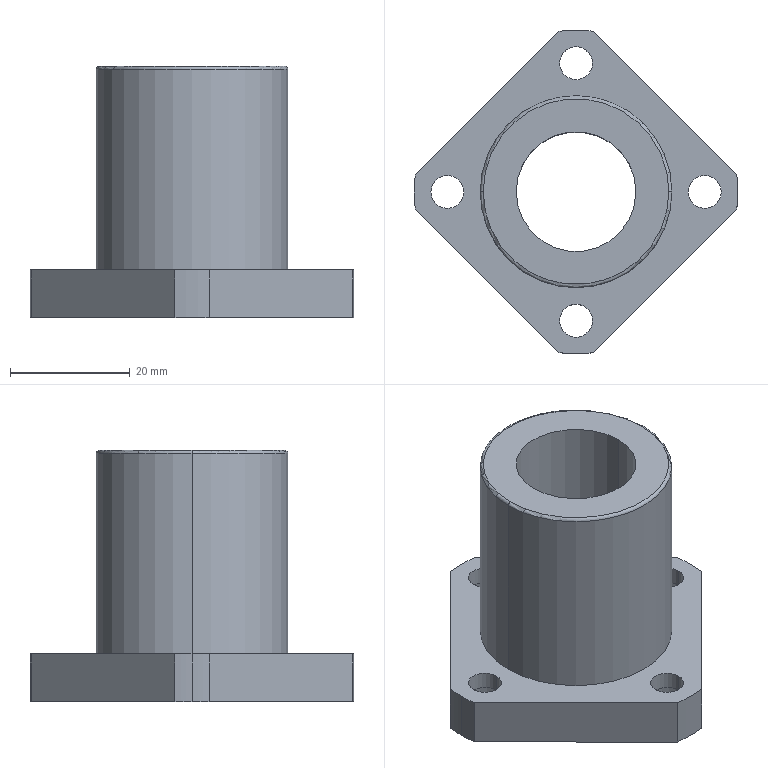Part | SolidWorks | features BaseBody 1 | 1 solid | 38 faces | box 54 x 54 x 42 mm | volume 26442 mm3 | cylinder 25 | plane 11 | torus 2 | commonest cylinder face diameters 5.5 x8 9 x8 54 x5 20 x2 32 x2
STEP:
#1=CARTESIAN_POINT('',(4.5,21.5,5.1));
#2=VERTEX_POINT('',#1);
#3=CARTESIAN_POINT('',(-4.5,21.5,5.1));
#4=VERTEX_POINT('',#3);
#5=CARTESIAN_POINT('',(0.,21.5,5.1));
#6=DIRECTION('',(0.,0.,-1.));
#7=DIRECTION('',(-1.,0.,0.));
#8=AXIS2_PLACEMENT_3D('',#5,#6,#7);
#9=CIRCLE('',#8,4.5);
#10=EDGE_CURVE('',#2,#4,#9,.T.);
#11=ORIENTED_EDGE('',*,*,#10,.F.);
#12=CARTESIAN_POINT('',(4.5,21.5,0.));
#13=VERTEX_POINT('',#12);
#14=CARTESIAN_POINT('',(4.5,21.5,0.));
#15=DIRECTION('',(0.,0.,-1.));
#16=VECTOR('',#15,1000.);
#17=LINE('',#14,#16);
#18=EDGE_CURVE('',#2,#13,#17,.T.);
#19=ORIENTED_EDGE('',*,*,#18,.T.);
#20=CARTESIAN_POINT('',(-4.5,21.5,0.));
#21=VERTEX_POINT('',#20);
#22=CARTESIAN_POINT('',(0.,21.5,0.));
#23=DIRECTION('',(0.,0.,-1.));
#24=DIRECTION('',(-1.,0.,0.));
#25=AXIS2_PLACEMENT_3D('',#22,#23,#24);
#26=CIRCLE('',#25,4.5);
#27=EDGE_CURVE('',#13,#21,#26,.T.);
#28=ORIENTED_EDGE('',*,*,#27,.T.);
#29=CARTESIAN_POINT('',(-4.5,21.5,0.));
#30=DIRECTION('',(0.,0.,-1.));
#31=VECTOR('',#30,1000.);
#32=LINE('',#29,#31);
#33=EDGE_CURVE('',#4,#21,#32,.T.);
#34=ORIENTED_EDGE('',*,*,#33,.F.);
#35=EDGE_LOOP('',(#11,#19,#28,#34));
#36=FACE_OUTER_BOUND('',#35,.T.);
#37=CARTESIAN_POINT('',(0.,21.5,0.));
#38=DIRECTION('',(0.,0.,-1.));
#39=DIRECTION('',(-1.,0.,0.));
#40=AXIS2_PLACEMENT_3D('',#37,#38,#39);
#41=CYLINDRICAL_SURFACE('',#40,4.5);
#42=ADVANCED_FACE('',(#36),#41,.F.);
#43=CARTESIAN_POINT('',(2.75,21.5,8.));
#44=VERTEX_POINT('',#43);
#45=CARTESIAN_POINT('',(-2.75,21.5,8.));
#46=VERTEX_POINT('',#45);
#47=CARTESIAN_POINT('',(0.,21.5,8.));
#48=DIRECTION('',(0.,0.,-1.));
#49=DIRECTION('',(-1.,0.,0.));
#50=AXIS2_PLACEMENT_3D('',#47,#48,#49);
#51=CIRCLE('',#50,2.75);
#52=EDGE_CURVE('',#44,#46,#51,.T.);
#53=ORIENTED_EDGE('',*,*,#52,.F.);
#54=CARTESIAN_POINT('',(2.75,21.5,5.1));
#55=VERTEX_POINT('',#54);
#56=CARTESIAN_POINT('',(2.75,21.5,0.));
#57=DIRECTION('',(0.,0.,-1.));
#58=VECTOR('',#57,1000.);
#59=LINE('',#56,#58);
#60=EDGE_CURVE('',#44,#55,#59,.T.);
#61=ORIENTED_EDGE('',*,*,#60,.T.);
#62=CARTESIAN_POINT('',(-2.75,21.5,5.1));
#63=VERTEX_POINT('',#62);
#64=CARTESIAN_POINT('',(0.,21.5,5.1));
#65=DIRECTION('',(0.,0.,-1.));
#66=DIRECTION('',(-1.,0.,0.));
#67=AXIS2_PLACEMENT_3D('',#64,#65,#66);
#68=CIRCLE('',#67,2.75);
#69=EDGE_CURVE('',#55,#63,#68,.T.);
#70=ORIENTED_EDGE('',*,*,#69,.T.);
#71=CARTESIAN_POINT('',(-2.75,21.5,0.));
#72=DIRECTION('',(0.,0.,-1.));
#73=VECTOR('',#72,1000.);
#74=LINE('',#71,#73);
#75=EDGE_CURVE('',#46,#63,#74,.T.);
#76=ORIENTED_EDGE('',*,*,#75,.F.);
#77=EDGE_LOOP('',(#53,#61,#70,#76));
#78=FACE_OUTER_BOUND('',#77,.T.);
#79=CARTESIAN_POINT('',(0.,21.5,0.));
#80=DIRECTION('',(0.,0.,-1.));
#81=DIRECTION('',(-1.,0.,0.));
#82=AXIS2_PLACEMENT_3D('',#79,#80,#81);
#83=CYLINDRICAL_SURFACE('',#82,2.75);
#84=ADVANCED_FACE('',(#78),#83,.F.);
#85=CARTESIAN_POINT('',(-2.75,-21.5,5.1));
#86=VERTEX_POINT('',#85);
#87=CARTESIAN_POINT('',(2.75,-21.5,5.1));
#88=VERTEX_POINT('',#87);
#89=CARTESIAN_POINT('',(0.,-21.5,5.1));
#90=DIRECTION('',(0.,0.,1.));
#91=DIRECTION('',(1.,0.,0.));
#92=AXIS2_PLACEMENT_3D('',#89,#90,#91);
#93=CIRCLE('',#92,2.75);
#94=EDGE_CURVE('',#86,#88,#93,.T.);
#95=ORIENTED_EDGE('',*,*,#94,.F.);
#96=CARTESIAN_POINT('',(-2.75,-21.5,8.));
#97=VERTEX_POINT('',#96);
#98=CARTESIAN_POINT('',(-2.75,-21.5,8.));
#99=DIRECTION('',(0.,0.,1.));
#100=VECTOR('',#99,1000.);
#101=LINE('',#98,#100);
#102=EDGE_CURVE('',#86,#97,#101,.T.);
#103=ORIENTED_EDGE('',*,*,#102,.T.);
#104=CARTESIAN_POINT('',(2.75,-21.5,8.));
#105=VERTEX_POINT('',#104);
#106=CARTESIAN_POINT('',(0.,-21.5,8.));
#107=DIRECTION('',(0.,0.,1.));
#108=DIRECTION('',(1.,0.,0.));
#109=AXIS2_PLACEMENT_3D('',#106,#107,#108);
#110=CIRCLE('',#109,2.75);
#111=EDGE_CURVE('',#97,#105,#110,.T.);
#112=ORIENTED_EDGE('',*,*,#111,.T.);
#113=CARTESIAN_POINT('',(2.75,-21.5,8.));
#114=DIRECTION('',(0.,0.,1.));
#115=VECTOR('',#114,1000.);
#116=LINE('',#113,#115);
#117=EDGE_CURVE('',#88,#105,#116,.T.);
#118=ORIENTED_EDGE('',*,*,#117,.F.);
#119=EDGE_LOOP('',(#95,#103,#112,#118));
#120=FACE_OUTER_BOUND('',#119,.T.);
#121=CARTESIAN_POINT('',(0.,-21.5,8.));
#122=DIRECTION('',(0.,0.,1.));
#123=DIRECTION('',(1.,0.,0.));
#124=AXIS2_PLACEMENT_3D('',#121,#122,#123);
#125=CYLINDRICAL_SURFACE('',#124,2.75);
#126=ADVANCED_FACE('',(#120),#125,.F.);
#127=CARTESIAN_POINT('',(-4.5,-21.5,0.));
#128=VERTEX_POINT('',#127);
#129=CARTESIAN_POINT('',(4.5,-21.5,0.));
#130=VERTEX_POINT('',#129);
#131=CARTESIAN_POINT('',(0.,-21.5,0.));
#132=DIRECTION('',(0.,0.,1.));
#133=DIRECTION('',(1.,0.,0.));
#134=AXIS2_PLACEMENT_3D('',#131,#132,#133);
#135=CIRCLE('',#134,4.5);
#136=EDGE_CURVE('',#128,#130,#135,.T.);
#137=ORIENTED_EDGE('',*,*,#136,.F.);
#138=CARTESIAN_POINT('',(-4.5,-21.5,5.1));
#139=VERTEX_POINT('',#138);
#140=CARTESIAN_POINT('',(-4.5,-21.5,8.));
#141=DIRECTION('',(0.,0.,1.));
#142=VECTOR('',#141,1000.);
#143=LINE('',#140,#142);
#144=EDGE_CURVE('',#128,#139,#143,.T.);
#145=ORIENTED_EDGE('',*,*,#144,.T.);
#146=CARTESIAN_POINT('',(4.5,-21.5,5.1));
#147=VERTEX_POINT('',#146);
#148=CARTESIAN_POINT('',(0.,-21.5,5.1));
#149=DIRECTION('',(0.,0.,1.));
#150=DIRECTION('',(1.,0.,0.));
#151=AXIS2_PLACEMENT_3D('',#148,#149,#150);
#152=CIRCLE('',#151,4.5);
#153=EDGE_CURVE('',#139,#147,#152,.T.);
#154=ORIENTED_EDGE('',*,*,#153,.T.);
#155=CARTESIAN_POINT('',(4.5,-21.5,8.));
#156=DIRECTION('',(0.,0.,1.));
#157=VECTOR('',#156,1000.);
#158=LINE('',#155,#157);
#159=EDGE_CURVE('',#130,#147,#158,.T.);
#160=ORIENTED_EDGE('',*,*,#159,.F.);
#161=EDGE_LOOP('',(#137,#145,#154,#160));
#162=FACE_OUTER_BOUND('',#161,.T.);
#163=CARTESIAN_POINT('',(0.,-21.5,8.));
#164=DIRECTION('',(0.,0.,1.));
#165=DIRECTION('',(1.,0.,0.));
#166=AXIS2_PLACEMENT_3D('',#163,#164,#165);
#167=CYLINDRICAL_SURFACE('',#166,4.5);
#168=ADVANCED_FACE('',(#162),#167,.F.);
#169=CARTESIAN_POINT('',(18.75,0.,5.1));
#170=VERTEX_POINT('',#169);
#171=CARTESIAN_POINT('',(24.25,0.,5.1));
#172=VERTEX_POINT('',#171);
#173=CARTESIAN_POINT('',(21.5,0.,5.1));
#174=DIRECTION('',(0.,0.,1.));
#175=DIRECTION('',(1.,0.,0.));
#176=AXIS2_PLACEMENT_3D('',#173,#174,#175);
#177=CIRCLE('',#176,2.75);
#178=EDGE_CURVE('',#170,#172,#177,.T.);
#179=ORIENTED_EDGE('',*,*,#178,.F.);
#180=CARTESIAN_POINT('',(18.75,0.,8.));
#181=VERTEX_POINT('',#180);
#182=CARTESIAN_POINT('',(18.75,0.,8.));
#183=DIRECTION('',(0.,0.,1.));
#184=VECTOR('',#183,1000.);
#185=LINE('',#182,#184);
#186=EDGE_CURVE('',#170,#181,#185,.T.);
#187=ORIENTED_EDGE('',*,*,#186,.T.);
#188=CARTESIAN_POINT('',(24.25,0.,8.));
#189=VERTEX_POINT('',#188);
#190=CARTESIAN_POINT('',(21.5,0.,8.));
#191=DIRECTION('',(0.,0.,1.));
#192=DIRECTION('',(1.,0.,0.));
#193=AXIS2_PLACEMENT_3D('',#190,#191,#192);
#194=CIRCLE('',#193,2.75);
#195=EDGE_CURVE('',#181,#189,#194,.T.);
#196=ORIENTED_EDGE('',*,*,#195,.T.);
#197=CARTESIAN_POINT('',(24.25,0.,8.));
#198=DIRECTION('',(0.,0.,1.));
#199=VECTOR('',#198,1000.);
#200=LINE('',#197,#199);
#201=EDGE_CURVE('',#172,#189,#200,.T.);
#202=ORIENTED_EDGE('',*,*,#201,.F.);
#203=EDGE_LOOP('',(#179,#187,#196,#202));
#204=FACE_OUTER_BOUND('',#203,.T.);
#205=CARTESIAN_POINT('',(21.5,0.,8.));
#206=DIRECTION('',(0.,0.,1.));
#207=DIRECTION('',(1.,0.,0.));
#208=AXIS2_PLACEMENT_3D('',#205,#206,#207);
#209=CYLINDRICAL_SURFACE('',#208,2.75);
#210=ADVANCED_FACE('',(#204),#209,.F.);
#211=CARTESIAN_POINT('',(17.,0.,0.));
#212=VERTEX_POINT('',#211);
#213=CARTESIAN_POINT('',(26.,0.,0.));
#214=VERTEX_POINT('',#213);
#215=CARTESIAN_POINT('',(21.5,0.,0.));
#216=DIRECTION('',(0.,0.,1.));
#217=DIRECTION('',(1.,0.,0.));
#218=AXIS2_PLACEMENT_3D('',#215,#216,#217);
#219=CIRCLE('',#218,4.5);
#220=EDGE_CURVE('',#212,#214,#219,.T.);
#221=ORIENTED_EDGE('',*,*,#220,.F.);
#222=CARTESIAN_POINT('',(17.,0.,5.1));
#223=VERTEX_POINT('',#222);
#224=CARTESIAN_POINT('',(17.,0.,8.));
#225=DIRECTION('',(0.,0.,1.));
#226=VECTOR('',#225,1000.);
#227=LINE('',#224,#226);
#228=EDGE_CURVE('',#212,#223,#227,.T.);
#229=ORIENTED_EDGE('',*,*,#228,.T.);
#230=CARTESIAN_POINT('',(26.,0.,5.1));
#231=VERTEX_POINT('',#230);
#232=CARTESIAN_POINT('',(21.5,0.,5.1));
#233=DIRECTION('',(0.,0.,1.));
#234=DIRECTION('',(1.,0.,0.));
#235=AXIS2_PLACEMENT_3D('',#232,#233,#234);
#236=CIRCLE('',#235,4.5);
#237=EDGE_CURVE('',#223,#231,#236,.T.);
#238=ORIENTED_EDGE('',*,*,#237,.T.);
#239=CARTESIAN_POINT('',(26.,0.,8.));
#240=DIRECTION('',(0.,0.,1.));
#241=VECTOR('',#240,1000.);
#242=LINE('',#239,#241);
#243=EDGE_CURVE('',#214,#231,#242,.T.);
#244=ORIENTED_EDGE('',*,*,#243,.F.);
#245=EDGE_LOOP('',(#221,#229,#238,#244));
#246=FACE_OUTER_BOUND('',#245,.T.);
#247=CARTESIAN_POINT('',(21.5,0.,8.));
#248=DIRECTION('',(0.,0.,1.));
#249=DIRECTION('',(1.,0.,0.));
#250=AXIS2_PLACEMENT_3D('',#247,#248,#249);
#251=CYLINDRICAL_SURFACE('',#250,4.5);
#252=ADVANCED_FACE('',(#246),#251,.F.);
#253=CARTESIAN_POINT('',(-17.,0.,5.1));
#254=VERTEX_POINT('',#253);
#255=CARTESIAN_POINT('',(-26.,0.,5.1));
#256=VERTEX_POINT('',#255);
#257=CARTESIAN_POINT('',(-21.5,0.,5.1));
#258=DIRECTION('',(0.,0.,-1.));
#259=DIRECTION('',(-1.,0.,0.));
#260=AXIS2_PLACEMENT_3D('',#257,#258,#259);
#261=CIRCLE('',#260,4.5);
#262=EDGE_CURVE('',#254,#256,#261,.T.);
#263=ORIENTED_EDGE('',*,*,#262,.F.);
#264=CARTESIAN_POINT('',(-17.,0.,0.));
#265=VERTEX_POINT('',#264);
#266=CARTESIAN_POINT('',(-17.,0.,0.));
#267=DIRECTION('',(0.,0.,-1.));
#268=VECTOR('',#267,1000.);
#269=LINE('',#266,#268);
#270=EDGE_CURVE('',#254,#265,#269,.T.);
#271=ORIENTED_EDGE('',*,*,#270,.T.);
#272=CARTESIAN_POINT('',(-26.,0.,0.));
#273=VERTEX_POINT('',#272);
#274=CARTESIAN_POINT('',(-21.5,0.,0.));
#275=DIRECTION('',(0.,0.,-1.));
#276=DIRECTION('',(-1.,0.,0.));
#277=AXIS2_PLACEMENT_3D('',#274,#275,#276);
#278=CIRCLE('',#277,4.5);
#279=EDGE_CURVE('',#265,#273,#278,.T.);
#280=ORIENTED_EDGE('',*,*,#279,.T.);
#281=CARTESIAN_POINT('',(-26.,0.,0.));
#282=DIRECTION('',(0.,0.,-1.));
#283=VECTOR('',#282,1000.);
#284=LINE('',#281,#283);
#285=EDGE_CURVE('',#256,#273,#284,.T.);
#286=ORIENTED_EDGE('',*,*,#285,.F.);
#287=EDGE_LOOP('',(#263,#271,#280,#286));
#288=FACE_OUTER_BOUND('',#287,.T.);
#289=CARTESIAN_POINT('',(-21.5,0.,0.));
#290=DIRECTION('',(0.,0.,-1.));
#291=DIRECTION('',(-1.,0.,0.));
#292=AXIS2_PLACEMENT_3D('',#289,#290,#291);
#293=CYLINDRICAL_SURFACE('',#292,4.5);
#294=ADVANCED_FACE('',(#288),#293,.F.);
#295=CARTESIAN_POINT('',(-18.75,0.,8.));
#296=VERTEX_POINT('',#295);
#297=CARTESIAN_POINT('',(-24.25,0.,8.));
#298=VERTEX_POINT('',#297);
#299=CARTESIAN_POINT('',(-21.5,0.,8.));
#300=DIRECTION('',(0.,0.,-1.));
#301=DIRECTION('',(-1.,0.,0.));
#302=AXIS2_PLACEMENT_3D('',#299,#300,#301);
#303=CIRCLE('',#302,2.75);
#304=EDGE_CURVE('',#296,#298,#303,.T.);
#305=ORIENTED_EDGE('',*,*,#304,.F.);
#306=CARTESIAN_POINT('',(-18.75,0.,5.1));
#307=VERTEX_POINT('',#306);
#308=CARTESIAN_POINT('',(-18.75,0.,0.));
#309=DIRECTION('',(0.,0.,-1.));
#310=VECTOR('',#309,1000.);
#311=LINE('',#308,#310);
#312=EDGE_CURVE('',#296,#307,#311,.T.);
#313=ORIENTED_EDGE('',*,*,#312,.T.);
#314=CARTESIAN_POINT('',(-24.25,0.,5.1));
#315=VERTEX_POINT('',#314);
#316=CARTESIAN_POINT('',(-21.5,0.,5.1));
#317=DIRECTION('',(0.,0.,-1.));
#318=DIRECTION('',(-1.,0.,0.));
#319=AXIS2_PLACEMENT_3D('',#316,#317,#318);
#320=CIRCLE('',#319,2.75);
#321=EDGE_CURVE('',#307,#315,#320,.T.);
#322=ORIENTED_EDGE('',*,*,#321,.T.);
#323=CARTESIAN_POINT('',(-24.25,0.,0.));
#324=DIRECTION('',(0.,0.,-1.));
#325=VECTOR('',#324,1000.);
#326=LINE('',#323,#325);
#327=EDGE_CURVE('',#298,#315,#326,.T.);
#328=ORIENTED_EDGE('',*,*,#327,.F.);
#329=EDGE_LOOP('',(#305,#313,#322,#328));
#330=FACE_OUTER_BOUND('',#329,.T.);
#331=CARTESIAN_POINT('',(-21.5,0.,0.));
#332=DIRECTION('',(0.,0.,-1.));
#333=DIRECTION('',(-1.,0.,0.));
#334=AXIS2_PLACEMENT_3D('',#331,#332,#333);
#335=CYLINDRICAL_SURFACE('',#334,2.75);
#336=ADVANCED_FACE('',(#330),#335,.F.);
#337=CARTESIAN_POINT('',(-27.,0.,8.));
#338=VERTEX_POINT('',#337);
#339=CARTESIAN_POINT('',(-26.849,-2.849,8.));
#340=VERTEX_POINT('',#339);
#341=CARTESIAN_POINT('',(0.,0.,8.));
#342=DIRECTION('',(0.,0.,1.));
#343=DIRECTION('',(1.,0.,0.));
#344=AXIS2_PLACEMENT_3D('',#341,#342,#343);
#345=CIRCLE('',#344,27.);
#346=EDGE_CURVE('',#338,#340,#345,.T.);
#347=ORIENTED_EDGE('',*,*,#346,.F.);
#348=CARTESIAN_POINT('',(-27.,0.,0.));
#349=VERTEX_POINT('',#348);
#350=CARTESIAN_POINT('',(-27.,0.,8.));
#351=DIRECTION('',(0.,0.,-1.));
#352=VECTOR('',#351,1000.);
#353=LINE('',#350,#352);
#354=EDGE_CURVE('',#338,#349,#353,.T.);
#355=ORIENTED_EDGE('',*,*,#354,.T.);
#356=CARTESIAN_POINT('',(-26.849,-2.849,0.));
#357=VERTEX_POINT('',#356);
#358=CARTESIAN_POINT('',(0.,0.,0.));
#359=DIRECTION('',(0.,0.,1.));
#360=DIRECTION('',(1.,0.,0.));
#361=AXIS2_PLACEMENT_3D('',#358,#359,#360);
#362=CIRCLE('',#361,27.);
#363=EDGE_CURVE('',#349,#357,#362,.T.);
#364=ORIENTED_EDGE('',*,*,#363,.T.);
#365=CARTESIAN_POINT('',(-26.849,-2.849,8.));
#366=DIRECTION('',(0.,0.,-1.));
#367=VECTOR('',#366,1000.);
#368=LINE('',#365,#367);
#369=EDGE_CURVE('',#340,#357,#368,.T.);
#370=ORIENTED_EDGE('',*,*,#369,.F.);
#371=EDGE_LOOP('',(#347,#355,#364,#370));
#372=FACE_OUTER_BOUND('',#371,.T.);
#373=CARTESIAN_POINT('',(0.,0.,8.));
#374=DIRECTION('',(0.,0.,-1.));
#375=DIRECTION('',(-1.,0.,0.));
#376=AXIS2_PLACEMENT_3D('',#373,#374,#375);
#377=CYLINDRICAL_SURFACE('',#376,27.);
#378=ADVANCED_FACE('',(#372),#377,.T.);
#379=CARTESIAN_POINT('',(10.,0.,42.));
#380=VERTEX_POINT('',#379);
#381=CARTESIAN_POINT('',(-10.,0.,42.));
#382=VERTEX_POINT('',#381);
#383=CARTESIAN_POINT('',(0.,0.,42.));
#384=DIRECTION('',(0.,0.,-1.));
#385=DIRECTION('',(-1.,0.,0.));
#386=AXIS2_PLACEMENT_3D('',#383,#384,#385);
#387=CIRCLE('',#386,10.);
#388=EDGE_CURVE('',#380,#382,#387,.T.);
#389=ORIENTED_EDGE('',*,*,#388,.F.);
#390=CARTESIAN_POINT('',(10.,0.,0.));
#391=VERTEX_POINT('',#390);
#392=CARTESIAN_POINT('',(10.,0.,0.));
#393=DIRECTION('',(0.,0.,-1.));
#394=VECTOR('',#393,1000.);
#395=LINE('',#392,#394);
#396=EDGE_CURVE('',#380,#391,#395,.T.);
#397=ORIENTED_EDGE('',*,*,#396,.T.);
#398=CARTESIAN_POINT('',(-10.,0.,0.));
#399=VERTEX_POINT('',#398);
#400=CARTESIAN_POINT('',(0.,0.,0.));
#401=DIRECTION('',(0.,0.,-1.));
#402=DIRECTION('',(-1.,0.,0.));
#403=AXIS2_PLACEMENT_3D('',#400,#401,#402);
#404=CIRCLE('',#403,10.);
#405=EDGE_CURVE('',#391,#399,#404,.T.);
#406=ORIENTED_EDGE('',*,*,#405,.T.);
#407=CARTESIAN_POINT('',(-10.,0.,0.));
#408=DIRECTION('',(0.,0.,-1.));
#409=VECTOR('',#408,1000.);
#410=LINE('',#407,#409);
#411=EDGE_CURVE('',#382,#399,#410,.T.);
#412=ORIENTED_EDGE('',*,*,#411,.F.);
#413=EDGE_LOOP('',(#389,#397,#406,#412));
#414=FACE_OUTER_BOUND('',#413,.T.);
#415=CARTESIAN_POINT('',(0.,0.,0.));
#416=DIRECTION('',(0.,0.,-1.));
#417=DIRECTION('',(-1.,0.,0.));
#418=AXIS2_PLACEMENT_3D('',#415,#416,#417);
#419=CYLINDRICAL_SURFACE('',#418,10.);
#420=ADVANCED_FACE('',(#414),#419,.F.);
#421=CARTESIAN_POINT('',(-15.5,0.,42.));
#422=VERTEX_POINT('',#421);
#423=CARTESIAN_POINT('',(15.5,0.,42.));
#424=VERTEX_POINT('',#423);
#425=CARTESIAN_POINT('',(0.,0.,42.));
#426=DIRECTION('',(0.,0.,-1.));
#427=DIRECTION('',(-1.,0.,0.));
#428=AXIS2_PLACEMENT_3D('',#425,#426,#427);
#429=CIRCLE('',#428,15.5);
#430=EDGE_CURVE('',#422,#424,#429,.T.);
#431=ORIENTED_EDGE('',*,*,#430,.T.);
#432=CARTESIAN_POINT('',(16.,0.,41.5));
#433=VERTEX_POINT('',#432);
#434=CARTESIAN_POINT('',(15.5,0.,41.5));
#435=DIRECTION('',(0.,1.,0.));
#436=DIRECTION('',(-1.,0.,0.));
#437=AXIS2_PLACEMENT_3D('',#434,#435,#436);
#438=CIRCLE('',#437,0.5);
#439=EDGE_CURVE('',#424,#433,#438,.T.);
#440=ORIENTED_EDGE('',*,*,#439,.T.);
#441=CARTESIAN_POINT('',(-16.,0.,41.5));
#442=VERTEX_POINT('',#441);
#443=CARTESIAN_POINT('',(0.,0.,41.5));
#444=DIRECTION('',(0.,0.,-1.));
#445=DIRECTION('',(-1.,0.,0.));
#446=AXIS2_PLACEMENT_3D('',#443,#444,#445);
#447=CIRCLE('',#446,16.);
#448=EDGE_CURVE('',#442,#433,#447,.T.);
#449=ORIENTED_EDGE('',*,*,#448,.F.);
#450=CARTESIAN_POINT('',(-15.5,0.,41.5));
#451=DIRECTION('',(0.,-1.,0.));
#452=DIRECTION('',(0.,0.,-1.));
#453=AXIS2_PLACEMENT_3D('',#450,#451,#452);
#454=CIRCLE('',#453,0.5);
#455=EDGE_CURVE('',#422,#442,#454,.T.);
#456=ORIENTED_EDGE('',*,*,#455,.F.);
#457=EDGE_LOOP('',(#431,#440,#449,#456));
#458=FACE_OUTER_BOUND('',#457,.T.);
#459=CARTESIAN_POINT('',(0.,0.,41.5));
#460=DIRECTION('',(0.,0.,-1.));
#461=DIRECTION('',(-1.,0.,0.));
#462=AXIS2_PLACEMENT_3D('',#459,#460,#461);
#463=TOROIDAL_SURFACE('',#462,15.5,0.5);
#464=ADVANCED_FACE('',(#458),#463,.T.);
#465=ORIENTED_EDGE('',*,*,#448,.T.);
#466=CARTESIAN_POINT('',(16.,0.,8.));
#467=VERTEX_POINT('',#466);
#468=CARTESIAN_POINT('',(16.,0.,0.));
#469=DIRECTION('',(0.,0.,-1.));
#470=VECTOR('',#469,1000.);
#471=LINE('',#468,#470);
#472=EDGE_CURVE('',#433,#467,#471,.T.);
#473=ORIENTED_EDGE('',*,*,#472,.T.);
#474=CARTESIAN_POINT('',(-16.,0.,8.));
#475=VERTEX_POINT('',#474);
#476=CARTESIAN_POINT('',(0.,0.,8.));
#477=DIRECTION('',(0.,0.,1.));
#478=DIRECTION('',(1.,0.,0.));
#479=AXIS2_PLACEMENT_3D('',#476,#477,#478);
#480=CIRCLE('',#479,16.);
#481=EDGE_CURVE('',#467,#475,#480,.T.);
#482=ORIENTED_EDGE('',*,*,#481,.T.);
#483=CARTESIAN_POINT('',(-16.,0.,0.));
#484=DIRECTION('',(0.,0.,-1.));
#485=VECTOR('',#484,1000.);
#486=LINE('',#483,#485);
#487=EDGE_CURVE('',#442,#475,#486,.T.);
#488=ORIENTED_EDGE('',*,*,#487,.F.);
#489=EDGE_LOOP('',(#465,#473,#482,#488));
#490=FACE_OUTER_BOUND('',#489,.T.);
#491=CARTESIAN_POINT('',(0.,0.,0.));
#492=DIRECTION('',(0.,0.,-1.));
#493=DIRECTION('',(-1.,0.,0.));
#494=AXIS2_PLACEMENT_3D('',#491,#492,#493);
#495=CYLINDRICAL_SURFACE('',#494,16.);
#496=ADVANCED_FACE('',(#490),#495,.T.);
#497=CARTESIAN_POINT('',(0.,21.5,5.1));
#498=DIRECTION('',(0.,0.,-1.));
#499=DIRECTION('',(-1.,0.,0.));
#500=AXIS2_PLACEMENT_3D('',#497,#498,#499);
#501=CIRCLE('',#500,2.75);
#502=EDGE_CURVE('',#63,#55,#501,.T.);
#503=ORIENTED_EDGE('',*,*,#502,.F.);
#504=ORIENTED_EDGE('',*,*,#69,.F.);
#505=EDGE_LOOP('',(#503,#504));
#506=FACE_BOUND('',#505,.T.);
#507=CARTESIAN_POINT('',(0.,21.5,5.1));
#508=DIRECTION('',(0.,0.,-1.));
#509=DIRECTION('',(-1.,0.,0.));
#510=AXIS2_PLACEMENT_3D('',#507,#508,#509);
#511=CIRCLE('',#510,4.5);
#512=EDGE_CURVE('',#4,#2,#511,.T.);
#513=ORIENTED_EDGE('',*,*,#512,.T.);
#514=ORIENTED_EDGE('',*,*,#10,.T.);
#515=EDGE_LOOP('',(#513,#514));
#516=FACE_OUTER_BOUND('',#515,.T.);
#517=CARTESIAN_POINT('',(0.,24.25,5.1));
#518=DIRECTION('',(0.,0.,-1.));
#519=DIRECTION('',(0.,-1.,0.));
#520=AXIS2_PLACEMENT_3D('',#517,#518,#519);
#521=PLANE('',#520);
#522=ADVANCED_FACE('',(#506,#516),#521,.T.);
#523=CARTESIAN_POINT('',(0.,-21.5,5.1));
#524=DIRECTION('',(0.,0.,1.));
#525=DIRECTION('',(1.,0.,0.));
#526=AXIS2_PLACEMENT_3D('',#523,#524,#525);
#527=CIRCLE('',#526,2.75);
#528=EDGE_CURVE('',#88,#86,#527,.T.);
#529=ORIENTED_EDGE('',*,*,#528,.T.);
#530=ORIENTED_EDGE('',*,*,#94,.T.);
#531=EDGE_LOOP('',(#529,#530));
#532=FACE_BOUND('',#531,.T.);
#533=CARTESIAN_POINT('',(0.,-21.5,5.1));
#534=DIRECTION('',(0.,0.,1.));
#535=DIRECTION('',(1.,0.,0.));
#536=AXIS2_PLACEMENT_3D('',#533,#534,#535);
#537=CIRCLE('',#536,4.5);
#538=EDGE_CURVE('',#147,#139,#537,.T.);
#539=ORIENTED_EDGE('',*,*,#538,.F.);
#540=ORIENTED_EDGE('',*,*,#153,.F.);
#541=EDGE_LOOP('',(#539,#540));
#542=FACE_OUTER_BOUND('',#541,.T.);
#543=CARTESIAN_POINT('',(0.,-26.,5.1));
#544=DIRECTION('',(0.,0.,-1.));
#545=DIRECTION('',(0.,-1.,0.));
#546=AXIS2_PLACEMENT_3D('',#543,#544,#545);
#547=PLANE('',#546);
#548=ADVANCED_FACE('',(#532,#542),#547,.T.);
#549=CARTESIAN_POINT('',(21.5,0.,5.1));
#550=DIRECTION('',(0.,0.,1.));
#551=DIRECTION('',(1.,0.,0.));
#552=AXIS2_PLACEMENT_3D('',#549,#550,#551);
#553=CIRCLE('',#552,2.75);
#554=EDGE_CURVE('',#172,#170,#553,.T.);
#555=ORIENTED_EDGE('',*,*,#554,.T.);
#556=ORIENTED_EDGE('',*,*,#178,.T.);
#557=EDGE_LOOP('',(#555,#556));
#558=FACE_BOUND('',#557,.T.);
#559=CARTESIAN_POINT('',(21.5,0.,5.1));
#560=DIRECTION('',(0.,0.,1.));
#561=DIRECTION('',(1.,0.,0.));
#562=AXIS2_PLACEMENT_3D('',#559,#560,#561);
#563=CIRCLE('',#562,4.5);
#564=EDGE_CURVE('',#231,#223,#563,.T.);
#565=ORIENTED_EDGE('',*,*,#564,.F.);
#566=ORIENTED_EDGE('',*,*,#237,.F.);
#567=EDGE_LOOP('',(#565,#566));
#568=FACE_OUTER_BOUND('',#567,.T.);
#569=CARTESIAN_POINT('',(26.,0.,5.1));
#570=DIRECTION('',(0.,0.,-1.));
#571=DIRECTION('',(0.,-1.,0.));
#572=AXIS2_PLACEMENT_3D('',#569,#570,#571);
#573=PLANE('',#572);
#574=ADVANCED_FACE('',(#558,#568),#573,.T.);
#575=CARTESIAN_POINT('',(-21.5,0.,5.1));
#576=DIRECTION('',(0.,0.,-1.));
#577=DIRECTION('',(-1.,0.,0.));
#578=AXIS2_PLACEMENT_3D('',#575,#576,#577);
#579=CIRCLE('',#578,2.75);
#580=EDGE_CURVE('',#315,#307,#579,.T.);
#581=ORIENTED_EDGE('',*,*,#580,.F.);
#582=ORIENTED_EDGE('',*,*,#321,.F.);
#583=EDGE_LOOP('',(#581,#582));
#584=FACE_BOUND('',#583,.T.);
#585=CARTESIAN_POINT('',(-21.5,0.,5.1));
#586=DIRECTION('',(0.,0.,-1.));
#587=DIRECTION('',(-1.,0.,0.));
#588=AXIS2_PLACEMENT_3D('',#585,#586,#587);
#589=CIRCLE('',#588,4.5);
#590=EDGE_CURVE('',#256,#254,#589,.T.);
#591=ORIENTED_EDGE('',*,*,#590,.T.);
#592=ORIENTED_EDGE('',*,*,#262,.T.);
#593=EDGE_LOOP('',(#591,#592));
#594=FACE_OUTER_BOUND('',#593,.T.);
#595=CARTESIAN_POINT('',(-24.25,0.,5.1));
#596=DIRECTION('',(0.,0.,-1.));
#597=DIRECTION('',(0.,-1.,0.));
#598=AXIS2_PLACEMENT_3D('',#595,#596,#597);
#599=PLANE('',#598);
#600=ADVANCED_FACE('',(#584,#594),#599,.T.);
#601=CARTESIAN_POINT('',(0.,0.,8.));
#602=DIRECTION('',(0.,0.,1.));
#603=DIRECTION('',(1.,0.,0.));
#604=AXIS2_PLACEMENT_3D('',#601,#602,#603);
#605=CIRCLE('',#604,16.);
#606=EDGE_CURVE('',#475,#467,#605,.T.);
#607=ORIENTED_EDGE('',*,*,#606,.F.);
#608=ORIENTED_EDGE('',*,*,#481,.F.);
#609=EDGE_LOOP('',(#607,#608));
#610=FACE_BOUND('',#609,.T.);
#611=CARTESIAN_POINT('',(-21.5,0.,8.));
#612=DIRECTION('',(0.,0.,-1.));
#613=DIRECTION('',(-1.,0.,0.));
#614=AXIS2_PLACEMENT_3D('',#611,#612,#613);
#615=CIRCLE('',#614,2.75);
#616=EDGE_CURVE('',#298,#296,#615,.T.);
#617=ORIENTED_EDGE('',*,*,#616,.T.);
#618=ORIENTED_EDGE('',*,*,#304,.T.);
#619=EDGE_LOOP('',(#617,#618));
#620=FACE_BOUND('',#619,.T.);
#621=CARTESIAN_POINT('',(21.5,0.,8.));
#622=DIRECTION('',(0.,0.,1.));
#623=DIRECTION('',(1.,0.,0.));
#624=AXIS2_PLACEMENT_3D('',#621,#622,#623);
#625=CIRCLE('',#624,2.75);
#626=EDGE_CURVE('',#189,#181,#625,.T.);
#627=ORIENTED_EDGE('',*,*,#626,.F.);
#628=ORIENTED_EDGE('',*,*,#195,.F.);
#629=EDGE_LOOP('',(#627,#628));
#630=FACE_BOUND('',#629,.T.);
#631=CARTESIAN_POINT('',(0.,-21.5,8.));
#632=DIRECTION('',(0.,0.,1.));
#633=DIRECTION('',(1.,0.,0.));
#634=AXIS2_PLACEMENT_3D('',#631,#632,#633);
#635=CIRCLE('',#634,2.75);
#636=EDGE_CURVE('',#105,#97,#635,.T.);
#637=ORIENTED_EDGE('',*,*,#636,.F.);
#638=ORIENTED_EDGE('',*,*,#111,.F.);
#639=EDGE_LOOP('',(#637,#638));
#640=FACE_BOUND('',#639,.T.);
#641=CARTESIAN_POINT('',(0.,21.5,8.));
#642=DIRECTION('',(0.,0.,-1.));
#643=DIRECTION('',(-1.,0.,0.));
#644=AXIS2_PLACEMENT_3D('',#641,#642,#643);
#645=CIRCLE('',#644,2.75);
#646=EDGE_CURVE('',#46,#44,#645,.T.);
#647=ORIENTED_EDGE('',*,*,#646,.T.);
#648=ORIENTED_EDGE('',*,*,#52,.T.);
#649=EDGE_LOOP('',(#647,#648));
#650=FACE_BOUND('',#649,.T.);
#651=CARTESIAN_POINT('',(-2.849,26.849,8.));
#652=VERTEX_POINT('',#651);
#653=CARTESIAN_POINT('',(-26.849,2.849,8.));
#654=VERTEX_POINT('',#653);
#655=CARTESIAN_POINT('',(-2.849,26.849,8.));
#656=DIRECTION('',(-0.7071,-0.7071,0.));
#657=VECTOR('',#656,1000.);
#658=LINE('',#655,#657);
#659=EDGE_CURVE('',#652,#654,#658,.T.);
#660=ORIENTED_EDGE('',*,*,#659,.T.);
#661=CARTESIAN_POINT('',(0.,0.,8.));
#662=DIRECTION('',(0.,0.,1.));
#663=DIRECTION('',(1.,0.,0.));
#664=AXIS2_PLACEMENT_3D('',#661,#662,#663);
#665=CIRCLE('',#664,27.);
#666=EDGE_CURVE('',#654,#338,#665,.T.);
#667=ORIENTED_EDGE('',*,*,#666,.T.);
#668=ORIENTED_EDGE('',*,*,#346,.T.);
#669=CARTESIAN_POINT('',(-2.849,-26.849,8.));
#670=VERTEX_POINT('',#669);
#671=CARTESIAN_POINT('',(-26.849,-2.849,8.));
#672=DIRECTION('',(0.7071,-0.7071,0.));
#673=VECTOR('',#672,1000.);
#674=LINE('',#671,#673);
#675=EDGE_CURVE('',#340,#670,#674,.T.);
#676=ORIENTED_EDGE('',*,*,#675,.T.);
#677=CARTESIAN_POINT('',(2.849,-26.849,8.));
#678=VERTEX_POINT('',#677);
#679=CARTESIAN_POINT('',(0.,0.,8.));
#680=DIRECTION('',(0.,0.,1.));
#681=DIRECTION('',(1.,0.,0.));
#682=AXIS2_PLACEMENT_3D('',#679,#680,#681);
#683=CIRCLE('',#682,27.);
#684=EDGE_CURVE('',#670,#678,#683,.T.);
#685=ORIENTED_EDGE('',*,*,#684,.T.);
#686=CARTESIAN_POINT('',(26.849,-2.849,8.));
#687=VERTEX_POINT('',#686);
#688=CARTESIAN_POINT('',(2.849,-26.849,8.));
#689=DIRECTION('',(0.7071,0.7071,0.));
#690=VECTOR('',#689,1000.);
#691=LINE('',#688,#690);
#692=EDGE_CURVE('',#678,#687,#691,.T.);
#693=ORIENTED_EDGE('',*,*,#692,.T.);
#694=CARTESIAN_POINT('',(26.849,2.849,8.));
#695=VERTEX_POINT('',#694);
#696=CARTESIAN_POINT('',(0.,0.,8.));
#697=DIRECTION('',(0.,0.,1.));
#698=DIRECTION('',(1.,0.,0.));
#699=AXIS2_PLACEMENT_3D('',#696,#697,#698);
#700=CIRCLE('',#699,27.);
#701=EDGE_CURVE('',#687,#695,#700,.T.);
#702=ORIENTED_EDGE('',*,*,#701,.T.);
#703=CARTESIAN_POINT('',(2.849,26.849,8.));
#704=VERTEX_POINT('',#703);
#705=CARTESIAN_POINT('',(26.849,2.849,8.));
#706=DIRECTION('',(-0.7071,0.7071,0.));
#707=VECTOR('',#706,1000.);
#708=LINE('',#705,#707);
#709=EDGE_CURVE('',#695,#704,#708,.T.);
#710=ORIENTED_EDGE('',*,*,#709,.T.);
#711=CARTESIAN_POINT('',(0.,0.,8.));
#712=DIRECTION('',(0.,0.,1.));
#713=DIRECTION('',(1.,0.,0.));
#714=AXIS2_PLACEMENT_3D('',#711,#712,#713);
#715=CIRCLE('',#714,27.);
#716=EDGE_CURVE('',#704,#652,#715,.T.);
#717=ORIENTED_EDGE('',*,*,#716,.T.);
#718=EDGE_LOOP('',(#660,#667,#668,#676,#685,#693,#702,#710,#717));
#719=FACE_OUTER_BOUND('',#718,.T.);
#720=CARTESIAN_POINT('',(0.,0.,8.));
#721=DIRECTION('',(0.,0.,1.));
#722=DIRECTION('',(1.,0.,0.));
#723=AXIS2_PLACEMENT_3D('',#720,#721,#722);
#724=PLANE('',#723);
#725=ADVANCED_FACE('',(#610,#620,#630,#640,#650,#719),#724,.T.);
#726=CARTESIAN_POINT('',(2.849,26.849,0.));
#727=VERTEX_POINT('',#726);
#728=CARTESIAN_POINT('',(-2.849,26.849,0.));
#729=VERTEX_POINT('',#728);
#730=CARTESIAN_POINT('',(0.,0.,0.));
#731=DIRECTION('',(0.,0.,1.));
#732=DIRECTION('',(1.,0.,0.));
#733=AXIS2_PLACEMENT_3D('',#730,#731,#732);
#734=CIRCLE('',#733,27.);
#735=EDGE_CURVE('',#727,#729,#734,.T.);
#736=ORIENTED_EDGE('',*,*,#735,.T.);
#737=CARTESIAN_POINT('',(-2.849,26.849,8.));
#738=DIRECTION('',(0.,0.,-1.));
#739=VECTOR('',#738,1000.);
#740=LINE('',#737,#739);
#741=EDGE_CURVE('',#652,#729,#740,.T.);
#742=ORIENTED_EDGE('',*,*,#741,.F.);
#743=ORIENTED_EDGE('',*,*,#716,.F.);
#744=CARTESIAN_POINT('',(2.849,26.849,8.));
#745=DIRECTION('',(0.,0.,-1.));
#746=VECTOR('',#745,1000.);
#747=LINE('',#744,#746);
#748=EDGE_CURVE('',#704,#727,#747,.T.);
#749=ORIENTED_EDGE('',*,*,#748,.T.);
#750=EDGE_LOOP('',(#736,#742,#743,#749));
#751=FACE_OUTER_BOUND('',#750,.T.);
#752=CARTESIAN_POINT('',(0.,0.,8.));
#753=DIRECTION('',(0.,0.,-1.));
#754=DIRECTION('',(-1.,0.,0.));
#755=AXIS2_PLACEMENT_3D('',#752,#753,#754);
#756=CYLINDRICAL_SURFACE('',#755,27.);
#757=ADVANCED_FACE('',(#751),#756,.T.);
#758=CARTESIAN_POINT('',(26.849,2.849,0.));
#759=VERTEX_POINT('',#758);
#760=CARTESIAN_POINT('',(26.849,2.849,0.));
#761=DIRECTION('',(-0.7071,0.7071,0.));
#762=VECTOR('',#761,1000.);
#763=LINE('',#760,#762);
#764=EDGE_CURVE('',#759,#727,#763,.T.);
#765=ORIENTED_EDGE('',*,*,#764,.T.);
#766=ORIENTED_EDGE('',*,*,#748,.F.);
#767=ORIENTED_EDGE('',*,*,#709,.F.);
#768=CARTESIAN_POINT('',(26.849,2.849,8.));
#769=DIRECTION('',(0.,0.,-1.));
#770=VECTOR('',#769,1000.);
#771=LINE('',#768,#770);
#772=EDGE_CURVE('',#695,#759,#771,.T.);
#773=ORIENTED_EDGE('',*,*,#772,.T.);
#774=EDGE_LOOP('',(#765,#766,#767,#773));
#775=FACE_OUTER_BOUND('',#774,.T.);
#776=CARTESIAN_POINT('',(26.849,2.849,8.));
#777=DIRECTION('',(-0.7071,-0.7071,0.));
#778=DIRECTION('',(-0.7071,0.7071,0.));
#779=AXIS2_PLACEMENT_3D('',#776,#777,#778);
#780=PLANE('',#779);
#781=ADVANCED_FACE('',(#775),#780,.F.);
#782=CARTESIAN_POINT('',(26.849,-2.849,0.));
#783=VERTEX_POINT('',#782);
#784=CARTESIAN_POINT('',(0.,0.,0.));
#785=DIRECTION('',(0.,0.,1.));
#786=DIRECTION('',(1.,0.,0.));
#787=AXIS2_PLACEMENT_3D('',#784,#785,#786);
#788=CIRCLE('',#787,27.);
#789=EDGE_CURVE('',#783,#759,#788,.T.);
#790=ORIENTED_EDGE('',*,*,#789,.T.);
#791=ORIENTED_EDGE('',*,*,#772,.F.);
#792=ORIENTED_EDGE('',*,*,#701,.F.);
#793=CARTESIAN_POINT('',(26.849,-2.849,8.));
#794=DIRECTION('',(0.,0.,-1.));
#795=VECTOR('',#794,1000.);
#796=LINE('',#793,#795);
#797=EDGE_CURVE('',#687,#783,#796,.T.);
#798=ORIENTED_EDGE('',*,*,#797,.T.);
#799=EDGE_LOOP('',(#790,#791,#792,#798));
#800=FACE_OUTER_BOUND('',#799,.T.);
#801=CARTESIAN_POINT('',(0.,0.,8.));
#802=DIRECTION('',(0.,0.,-1.));
#803=DIRECTION('',(-1.,0.,0.));
#804=AXIS2_PLACEMENT_3D('',#801,#802,#803);
#805=CYLINDRICAL_SURFACE('',#804,27.);
#806=ADVANCED_FACE('',(#800),#805,.T.);
#807=CARTESIAN_POINT('',(2.849,-26.849,0.));
#808=VERTEX_POINT('',#807);
#809=CARTESIAN_POINT('',(2.849,-26.849,0.));
#810=DIRECTION('',(0.7071,0.7071,0.));
#811=VECTOR('',#810,1000.);
#812=LINE('',#809,#811);
#813=EDGE_CURVE('',#808,#783,#812,.T.);
#814=ORIENTED_EDGE('',*,*,#813,.T.);
#815=ORIENTED_EDGE('',*,*,#797,.F.);
#816=ORIENTED_EDGE('',*,*,#692,.F.);
#817=CARTESIAN_POINT('',(2.849,-26.849,8.));
#818=DIRECTION('',(0.,0.,-1.));
#819=VECTOR('',#818,1000.);
#820=LINE('',#817,#819);
#821=EDGE_CURVE('',#678,#808,#820,.T.);
#822=ORIENTED_EDGE('',*,*,#821,.T.);
#823=EDGE_LOOP('',(#814,#815,#816,#822));
#824=FACE_OUTER_BOUND('',#823,.T.);
#825=CARTESIAN_POINT('',(2.849,-26.849,8.));
#826=DIRECTION('',(-0.7071,0.7071,0.));
#827=DIRECTION('',(0.,0.,1.));
#828=AXIS2_PLACEMENT_3D('',#825,#826,#827);
#829=PLANE('',#828);
#830=ADVANCED_FACE('',(#824),#829,.F.);
#831=CARTESIAN_POINT('',(-2.849,-26.849,0.));
#832=VERTEX_POINT('',#831);
#833=CARTESIAN_POINT('',(0.,0.,0.));
#834=DIRECTION('',(0.,0.,1.));
#835=DIRECTION('',(1.,0.,0.));
#836=AXIS2_PLACEMENT_3D('',#833,#834,#835);
#837=CIRCLE('',#836,27.);
#838=EDGE_CURVE('',#832,#808,#837,.T.);
#839=ORIENTED_EDGE('',*,*,#838,.T.);
#840=ORIENTED_EDGE('',*,*,#821,.F.);
#841=ORIENTED_EDGE('',*,*,#684,.F.);
#842=CARTESIAN_POINT('',(-2.849,-26.849,8.));
#843=DIRECTION('',(0.,0.,-1.));
#844=VECTOR('',#843,1000.);
#845=LINE('',#842,#844);
#846=EDGE_CURVE('',#670,#832,#845,.T.);
#847=ORIENTED_EDGE('',*,*,#846,.T.);
#848=EDGE_LOOP('',(#839,#840,#841,#847));
#849=FACE_OUTER_BOUND('',#848,.T.);
#850=CARTESIAN_POINT('',(0.,0.,8.));
#851=DIRECTION('',(0.,0.,-1.));
#852=DIRECTION('',(-1.,0.,0.));
#853=AXIS2_PLACEMENT_3D('',#850,#851,#852);
#854=CYLINDRICAL_SURFACE('',#853,27.);
#855=ADVANCED_FACE('',(#849),#854,.T.);
#856=CARTESIAN_POINT('',(-26.849,-2.849,0.));
#857=DIRECTION('',(0.7071,-0.7071,0.));
#858=VECTOR('',#857,1000.);
#859=LINE('',#856,#858);
#860=EDGE_CURVE('',#357,#832,#859,.T.);
#861=ORIENTED_EDGE('',*,*,#860,.T.);
#862=ORIENTED_EDGE('',*,*,#846,.F.);
#863=ORIENTED_EDGE('',*,*,#675,.F.);
#864=ORIENTED_EDGE('',*,*,#369,.T.);
#865=EDGE_LOOP('',(#861,#862,#863,#864));
#866=FACE_OUTER_BOUND('',#865,.T.);
#867=CARTESIAN_POINT('',(-26.849,-2.849,8.));
#868=DIRECTION('',(0.7071,0.7071,0.));
#869=DIRECTION('',(0.,0.,-1.));
#870=AXIS2_PLACEMENT_3D('',#867,#868,#869);
#871=PLANE('',#870);
#872=ADVANCED_FACE('',(#866),#871,.F.);
#873=CARTESIAN_POINT('',(-26.849,2.849,0.));
#874=VERTEX_POINT('',#873);
#875=CARTESIAN_POINT('',(-2.849,26.849,0.));
#876=DIRECTION('',(-0.7071,-0.7071,0.));
#877=VECTOR('',#876,1000.);
#878=LINE('',#875,#877);
#879=EDGE_CURVE('',#729,#874,#878,.T.);
#880=ORIENTED_EDGE('',*,*,#879,.T.);
#881=CARTESIAN_POINT('',(-26.849,2.849,8.));
#882=DIRECTION('',(0.,0.,-1.));
#883=VECTOR('',#882,1000.);
#884=LINE('',#881,#883);
#885=EDGE_CURVE('',#654,#874,#884,.T.);
#886=ORIENTED_EDGE('',*,*,#885,.F.);
#887=ORIENTED_EDGE('',*,*,#659,.F.);
#888=ORIENTED_EDGE('',*,*,#741,.T.);
#889=EDGE_LOOP('',(#880,#886,#887,#888));
#890=FACE_OUTER_BOUND('',#889,.T.);
#891=CARTESIAN_POINT('',(-2.849,26.849,8.));
#892=DIRECTION('',(0.7071,-0.7071,0.));
#893=DIRECTION('',(0.,0.,-1.));
#894=AXIS2_PLACEMENT_3D('',#891,#892,#893);
#895=PLANE('',#894);
#896=ADVANCED_FACE('',(#890),#895,.F.);
#897=CARTESIAN_POINT('',(0.,0.,42.));
#898=DIRECTION('',(0.,0.,-1.));
#899=DIRECTION('',(-1.,0.,0.));
#900=AXIS2_PLACEMENT_3D('',#897,#898,#899);
#901=CIRCLE('',#900,10.);
#902=EDGE_CURVE('',#382,#380,#901,.T.);
#903=ORIENTED_EDGE('',*,*,#902,.T.);
#904=ORIENTED_EDGE('',*,*,#388,.T.);
#905=EDGE_LOOP('',(#903,#904));
#906=FACE_BOUND('',#905,.T.);
#907=ORIENTED_EDGE('',*,*,#430,.F.);
#908=CARTESIAN_POINT('',(0.,0.,42.));
#909=DIRECTION('',(0.,0.,-1.));
#910=DIRECTION('',(-1.,0.,0.));
#911=AXIS2_PLACEMENT_3D('',#908,#909,#910);
#912=CIRCLE('',#911,15.5);
#913=EDGE_CURVE('',#424,#422,#912,.T.);
#914=ORIENTED_EDGE('',*,*,#913,.F.);
#915=EDGE_LOOP('',(#907,#914));
#916=FACE_OUTER_BOUND('',#915,.T.);
#917=CARTESIAN_POINT('',(-15.5,0.,42.));
#918=DIRECTION('',(0.,0.,1.));
#919=DIRECTION('',(0.,-1.,0.));
#920=AXIS2_PLACEMENT_3D('',#917,#918,#919);
#921=PLANE('',#920);
#922=ADVANCED_FACE('',(#906,#916),#921,.T.);
#923=CARTESIAN_POINT('',(0.,0.,0.));
#924=DIRECTION('',(0.,0.,-1.));
#925=DIRECTION('',(-1.,0.,0.));
#926=AXIS2_PLACEMENT_3D('',#923,#924,#925);
#927=CIRCLE('',#926,10.);
#928=EDGE_CURVE('',#399,#391,#927,.T.);
#929=ORIENTED_EDGE('',*,*,#928,.F.);
#930=ORIENTED_EDGE('',*,*,#405,.F.);
#931=EDGE_LOOP('',(#929,#930));
#932=FACE_BOUND('',#931,.T.);
#933=CARTESIAN_POINT('',(-21.5,0.,0.));
#934=DIRECTION('',(0.,0.,-1.));
#935=DIRECTION('',(-1.,0.,0.));
#936=AXIS2_PLACEMENT_3D('',#933,#934,#935);
#937=CIRCLE('',#936,4.5);
#938=EDGE_CURVE('',#273,#265,#937,.T.);
#939=ORIENTED_EDGE('',*,*,#938,.F.);
#940=ORIENTED_EDGE('',*,*,#279,.F.);
#941=EDGE_LOOP('',(#939,#940));
#942=FACE_BOUND('',#941,.T.);
#943=CARTESIAN_POINT('',(21.5,0.,0.));
#944=DIRECTION('',(0.,0.,1.));
#945=DIRECTION('',(1.,0.,0.));
#946=AXIS2_PLACEMENT_3D('',#943,#944,#945);
#947=CIRCLE('',#946,4.5);
#948=EDGE_CURVE('',#214,#212,#947,.T.);
#949=ORIENTED_EDGE('',*,*,#948,.T.);
#950=ORIENTED_EDGE('',*,*,#220,.T.);
#951=EDGE_LOOP('',(#949,#950));
#952=FACE_BOUND('',#951,.T.);
#953=CARTESIAN_POINT('',(0.,-21.5,0.));
#954=DIRECTION('',(0.,0.,1.));
#955=DIRECTION('',(1.,0.,0.));
#956=AXIS2_PLACEMENT_3D('',#953,#954,#955);
#957=CIRCLE('',#956,4.5);
#958=EDGE_CURVE('',#130,#128,#957,.T.);
#959=ORIENTED_EDGE('',*,*,#958,.T.);
#960=ORIENTED_EDGE('',*,*,#136,.T.);
#961=EDGE_LOOP('',(#959,#960));
#962=FACE_BOUND('',#961,.T.);
#963=CARTESIAN_POINT('',(0.,21.5,0.));
#964=DIRECTION('',(0.,0.,-1.));
#965=DIRECTION('',(-1.,0.,0.));
#966=AXIS2_PLACEMENT_3D('',#963,#964,#965);
#967=CIRCLE('',#966,4.5);
#968=EDGE_CURVE('',#21,#13,#967,.T.);
#969=ORIENTED_EDGE('',*,*,#968,.F.);
#970=ORIENTED_EDGE('',*,*,#27,.F.);
#971=EDGE_LOOP('',(#969,#970));
#972=FACE_BOUND('',#971,.T.);
#973=ORIENTED_EDGE('',*,*,#879,.F.);
#974=ORIENTED_EDGE('',*,*,#735,.F.);
#975=ORIENTED_EDGE('',*,*,#764,.F.);
#976=ORIENTED_EDGE('',*,*,#789,.F.);
#977=ORIENTED_EDGE('',*,*,#813,.F.);
#978=ORIENTED_EDGE('',*,*,#838,.F.);
#979=ORIENTED_EDGE('',*,*,#860,.F.);
#980=ORIENTED_EDGE('',*,*,#363,.F.);
#981=CARTESIAN_POINT('',(0.,0.,0.));
#982=DIRECTION('',(0.,0.,1.));
#983=DIRECTION('',(1.,0.,0.));
#984=AXIS2_PLACEMENT_3D('',#981,#982,#983);
#985=CIRCLE('',#984,27.);
#986=EDGE_CURVE('',#874,#349,#985,.T.);
#987=ORIENTED_EDGE('',*,*,#986,.F.);
#988=EDGE_LOOP('',(#973,#974,#975,#976,#977,#978,#979,#980,#987));
#989=FACE_OUTER_BOUND('',#988,.T.);
#990=CARTESIAN_POINT('',(-10.,0.,0.));
#991=DIRECTION('',(0.,0.,-1.));
#992=DIRECTION('',(0.,-1.,0.));
#993=AXIS2_PLACEMENT_3D('',#990,#991,#992);
#994=PLANE('',#993);
#995=ADVANCED_FACE('',(#932,#942,#952,#962,#972,#989),#994,.T.);
#996=ORIENTED_EDGE('',*,*,#472,.F.);
#997=CARTESIAN_POINT('',(0.,0.,41.5));
#998=DIRECTION('',(0.,0.,-1.));
#999=DIRECTION('',(-1.,0.,0.));
#1000=AXIS2_PLACEMENT_3D('',#997,#998,#999);
#1001=CIRCLE('',#1000,16.);
#1002=EDGE_CURVE('',#433,#442,#1001,.T.);
#1003=ORIENTED_EDGE('',*,*,#1002,.T.);
#1004=ORIENTED_EDGE('',*,*,#487,.T.);
#1005=ORIENTED_EDGE('',*,*,#606,.T.);
#1006=EDGE_LOOP('',(#996,#1003,#1004,#1005));
#1007=FACE_OUTER_BOUND('',#1006,.T.);
#1008=CARTESIAN_POINT('',(0.,0.,0.));
#1009=DIRECTION('',(0.,0.,-1.));
#1010=DIRECTION('',(-1.,0.,0.));
#1011=AXIS2_PLACEMENT_3D('',#1008,#1009,#1010);
#1012=CYLINDRICAL_SURFACE('',#1011,16.);
#1013=ADVANCED_FACE('',(#1007),#1012,.T.);
#1014=ORIENTED_EDGE('',*,*,#439,.F.);
#1015=ORIENTED_EDGE('',*,*,#913,.T.);
#1016=ORIENTED_EDGE('',*,*,#455,.T.);
#1017=ORIENTED_EDGE('',*,*,#1002,.F.);
#1018=EDGE_LOOP('',(#1014,#1015,#1016,#1017));
#1019=FACE_OUTER_BOUND('',#1018,.T.);
#1020=CARTESIAN_POINT('',(0.,0.,41.5));
#1021=DIRECTION('',(0.,0.,-1.));
#1022=DIRECTION('',(-1.,0.,0.));
#1023=AXIS2_PLACEMENT_3D('',#1020,#1021,#1022);
#1024=TOROIDAL_SURFACE('',#1023,15.5,0.5);
#1025=ADVANCED_FACE('',(#1019),#1024,.T.);
#1026=ORIENTED_EDGE('',*,*,#396,.F.);
#1027=ORIENTED_EDGE('',*,*,#902,.F.);
#1028=ORIENTED_EDGE('',*,*,#411,.T.);
#1029=ORIENTED_EDGE('',*,*,#928,.T.);
#1030=EDGE_LOOP('',(#1026,#1027,#1028,#1029));
#1031=FACE_OUTER_BOUND('',#1030,.T.);
#1032=CARTESIAN_POINT('',(0.,0.,0.));
#1033=DIRECTION('',(0.,0.,-1.));
#1034=DIRECTION('',(-1.,0.,0.));
#1035=AXIS2_PLACEMENT_3D('',#1032,#1033,#1034);
#1036=CYLINDRICAL_SURFACE('',#1035,10.);
#1037=ADVANCED_FACE('',(#1031),#1036,.F.);
#1038=ORIENTED_EDGE('',*,*,#354,.F.);
#1039=ORIENTED_EDGE('',*,*,#666,.F.);
#1040=ORIENTED_EDGE('',*,*,#885,.T.);
#1041=ORIENTED_EDGE('',*,*,#986,.T.);
#1042=EDGE_LOOP('',(#1038,#1039,#1040,#1041));
#1043=FACE_OUTER_BOUND('',#1042,.T.);
#1044=CARTESIAN_POINT('',(0.,0.,8.));
#1045=DIRECTION('',(0.,0.,-1.));
#1046=DIRECTION('',(-1.,0.,0.));
#1047=AXIS2_PLACEMENT_3D('',#1044,#1045,#1046);
#1048=CYLINDRICAL_SURFACE('',#1047,27.);
#1049=ADVANCED_FACE('',(#1043),#1048,.T.);
#1050=ORIENTED_EDGE('',*,*,#312,.F.);
#1051=ORIENTED_EDGE('',*,*,#616,.F.);
#1052=ORIENTED_EDGE('',*,*,#327,.T.);
#1053=ORIENTED_EDGE('',*,*,#580,.T.);
#1054=EDGE_LOOP('',(#1050,#1051,#1052,#1053));
#1055=FACE_OUTER_BOUND('',#1054,.T.);
#1056=CARTESIAN_POINT('',(-21.5,0.,0.));
#1057=DIRECTION('',(0.,0.,-1.));
#1058=DIRECTION('',(-1.,0.,0.));
#1059=AXIS2_PLACEMENT_3D('',#1056,#1057,#1058);
#1060=CYLINDRICAL_SURFACE('',#1059,2.75);
#1061=ADVANCED_FACE('',(#1055),#1060,.F.);
#1062=ORIENTED_EDGE('',*,*,#270,.F.);
#1063=ORIENTED_EDGE('',*,*,#590,.F.);
#1064=ORIENTED_EDGE('',*,*,#285,.T.);
#1065=ORIENTED_EDGE('',*,*,#938,.T.);
#1066=EDGE_LOOP('',(#1062,#1063,#1064,#1065));
#1067=FACE_OUTER_BOUND('',#1066,.T.);
#1068=CARTESIAN_POINT('',(-21.5,0.,0.));
#1069=DIRECTION('',(0.,0.,-1.));
#1070=DIRECTION('',(-1.,0.,0.));
#1071=AXIS2_PLACEMENT_3D('',#1068,#1069,#1070);
#1072=CYLINDRICAL_SURFACE('',#1071,4.5);
#1073=ADVANCED_FACE('',(#1067),#1072,.F.);
#1074=ORIENTED_EDGE('',*,*,#228,.F.);
#1075=ORIENTED_EDGE('',*,*,#948,.F.);
#1076=ORIENTED_EDGE('',*,*,#243,.T.);
#1077=ORIENTED_EDGE('',*,*,#564,.T.);
#1078=EDGE_LOOP('',(#1074,#1075,#1076,#1077));
#1079=FACE_OUTER_BOUND('',#1078,.T.);
#1080=CARTESIAN_POINT('',(21.5,0.,8.));
#1081=DIRECTION('',(0.,0.,1.));
#1082=DIRECTION('',(1.,0.,0.));
#1083=AXIS2_PLACEMENT_3D('',#1080,#1081,#1082);
#1084=CYLINDRICAL_SURFACE('',#1083,4.5);
#1085=ADVANCED_FACE('',(#1079),#1084,.F.);
#1086=ORIENTED_EDGE('',*,*,#186,.F.);
#1087=ORIENTED_EDGE('',*,*,#554,.F.);
#1088=ORIENTED_EDGE('',*,*,#201,.T.);
#1089=ORIENTED_EDGE('',*,*,#626,.T.);
#1090=EDGE_LOOP('',(#1086,#1087,#1088,#1089));
#1091=FACE_OUTER_BOUND('',#1090,.T.);
#1092=CARTESIAN_POINT('',(21.5,0.,8.));
#1093=DIRECTION('',(0.,0.,1.));
#1094=DIRECTION('',(1.,0.,0.));
#1095=AXIS2_PLACEMENT_3D('',#1092,#1093,#1094);
#1096=CYLINDRICAL_SURFACE('',#1095,2.75);
#1097=ADVANCED_FACE('',(#1091),#1096,.F.);
#1098=ORIENTED_EDGE('',*,*,#144,.F.);
#1099=ORIENTED_EDGE('',*,*,#958,.F.);
#1100=ORIENTED_EDGE('',*,*,#159,.T.);
#1101=ORIENTED_EDGE('',*,*,#538,.T.);
#1102=EDGE_LOOP('',(#1098,#1099,#1100,#1101));
#1103=FACE_OUTER_BOUND('',#1102,.T.);
#1104=CARTESIAN_POINT('',(0.,-21.5,8.));
#1105=DIRECTION('',(0.,0.,1.));
#1106=DIRECTION('',(1.,0.,0.));
#1107=AXIS2_PLACEMENT_3D('',#1104,#1105,#1106);
#1108=CYLINDRICAL_SURFACE('',#1107,4.5);
#1109=ADVANCED_FACE('',(#1103),#1108,.F.);
#1110=ORIENTED_EDGE('',*,*,#102,.F.);
#1111=ORIENTED_EDGE('',*,*,#528,.F.);
#1112=ORIENTED_EDGE('',*,*,#117,.T.);
#1113=ORIENTED_EDGE('',*,*,#636,.T.);
#1114=EDGE_LOOP('',(#1110,#1111,#1112,#1113));
#1115=FACE_OUTER_BOUND('',#1114,.T.);
#1116=CARTESIAN_POINT('',(0.,-21.5,8.));
#1117=DIRECTION('',(0.,0.,1.));
#1118=DIRECTION('',(1.,0.,0.));
#1119=AXIS2_PLACEMENT_3D('',#1116,#1117,#1118);
#1120=CYLINDRICAL_SURFACE('',#1119,2.75);
#1121=ADVANCED_FACE('',(#1115),#1120,.F.);
#1122=ORIENTED_EDGE('',*,*,#60,.F.);
#1123=ORIENTED_EDGE('',*,*,#646,.F.);
#1124=ORIENTED_EDGE('',*,*,#75,.T.);
#1125=ORIENTED_EDGE('',*,*,#502,.T.);
#1126=EDGE_LOOP('',(#1122,#1123,#1124,#1125));
#1127=FACE_OUTER_BOUND('',#1126,.T.);
#1128=CARTESIAN_POINT('',(0.,21.5,0.));
#1129=DIRECTION('',(0.,0.,-1.));
#1130=DIRECTION('',(-1.,0.,0.));
#1131=AXIS2_PLACEMENT_3D('',#1128,#1129,#1130);
#1132=CYLINDRICAL_SURFACE('',#1131,2.75);
#1133=ADVANCED_FACE('',(#1127),#1132,.F.);
#1134=ORIENTED_EDGE('',*,*,#18,.F.);
#1135=ORIENTED_EDGE('',*,*,#512,.F.);
#1136=ORIENTED_EDGE('',*,*,#33,.T.);
#1137=ORIENTED_EDGE('',*,*,#968,.T.);
#1138=EDGE_LOOP('',(#1134,#1135,#1136,#1137));
#1139=FACE_OUTER_BOUND('',#1138,.T.);
#1140=CARTESIAN_POINT('',(0.,21.5,0.));
#1141=DIRECTION('',(0.,0.,-1.));
#1142=DIRECTION('',(-1.,0.,0.));
#1143=AXIS2_PLACEMENT_3D('',#1140,#1141,#1142);
#1144=CYLINDRICAL_SURFACE('',#1143,4.5);
#1145=ADVANCED_FACE('',(#1139),#1144,.F.);
#1146=CLOSED_SHELL('',(#42,#84,#126,#168,#210,#252,#294,#336,#378,#420,#464,#496,#522,#548,#574,#600,#725,#757,#781,#806,#830,#855,#872,#896,#922,#995,#1013,#1025,#1037,#1049,#1061,#1073,#1085,#1097,#1109,#1121,#1133,#1145));
#1147=MANIFOLD_SOLID_BREP('',#1146);
#1148=CARTESIAN_POINT('',(0.,0.,0.));
#1149=DIRECTION('',(0.,0.,1.));
#1150=DIRECTION('',(1.,0.,0.));
#1151=AXIS2_PLACEMENT_3D('',#1148,#1149,#1150);
#1152=(LENGTH_UNIT()NAMED_UNIT(*)SI_UNIT(.MILLI.,.METRE.));
#1153=UNCERTAINTY_MEASURE_WITH_UNIT(LENGTH_MEASURE(0.00001),#1152,'','');
#1154=(NAMED_UNIT(*)PLANE_ANGLE_UNIT()SI_UNIT($,.RADIAN.));
#1155=(NAMED_UNIT(*)SI_UNIT($,.STERADIAN.)SOLID_ANGLE_UNIT());
#1156=(GEOMETRIC_REPRESENTATION_CONTEXT(3)GLOBAL_UNCERTAINTY_ASSIGNED_CONTEXT((#1153))GLOBAL_UNIT_ASSIGNED_CONTEXT((#1152,#1154,#1155))REPRESENTATION_CONTEXT('',''));
#1157=ADVANCED_BREP_SHAPE_REPRESENTATION('',(#1147,#1151),#1156);